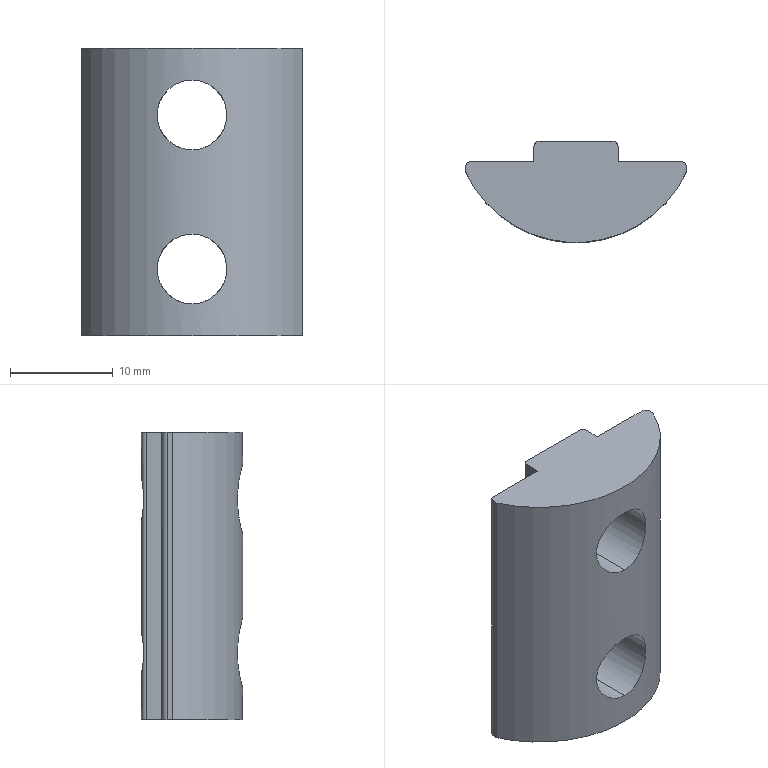Part | STEP file | 31E-01040QY25 | 1 solid | 24 faces | box 21.5 x 9.856 x 28 mm | volume 3296 mm3 | plane 11 | cylinder 9 | cone 4 | commonest cylinder face diameters 1 x4 6.8 x4 23.712 x1
STEP:
#1=CARTESIAN_POINT('',(15.532,8.15,3.1));
#2=VERTEX_POINT('',#1);
#3=CARTESIAN_POINT('',(15.532,8.15,9.9));
#4=VERTEX_POINT('',#3);
#5=CARTESIAN_POINT('',(15.532,8.15,6.5));
#6=DIRECTION('',(0.,1.,0.));
#7=AXIS2_PLACEMENT_3D('',#5,#6,$);
#8=CIRCLE('',#7,3.4);
#9=EDGE_CURVE('',#2,#4,#8,.T.);
#10=ORIENTED_EDGE('',*,*,#9,.F.);
#11=CARTESIAN_POINT('',(15.532,9.,2.25));
#12=VERTEX_POINT('',#11);
#13=CARTESIAN_POINT('',(15.532,353560.266,-353549.016));
#14=DIRECTION('',(0.,0.7071,-0.7071));
#15=VECTOR('',#14,1.);
#16=LINE('',#13,#15);
#17=EDGE_CURVE('',#2,#12,#16,.T.);
#18=ORIENTED_EDGE('',*,*,#17,.T.);
#19=CARTESIAN_POINT('',(11.932,9.,4.241));
#20=VERTEX_POINT('',#19);
#21=CARTESIAN_POINT('',(15.532,9.,6.5));
#22=DIRECTION('',(0.,1.,0.));
#23=AXIS2_PLACEMENT_3D('',#21,#22,$);
#24=CIRCLE('',#23,4.25);
#25=EDGE_CURVE('',#12,#20,#24,.T.);
#26=ORIENTED_EDGE('',*,*,#25,.T.);
#27=CARTESIAN_POINT('',(11.932,9.,8.759));
#28=VERTEX_POINT('',#27);
#29=CARTESIAN_POINT('',(11.932,9.,4.241));
#30=CARTESIAN_POINT('',(11.905,9.,4.284));
#31=CARTESIAN_POINT('',(11.88,8.998,4.329));
#32=CARTESIAN_POINT('',(11.857,8.995,4.375));
#33=CARTESIAN_POINT('',(11.806,8.986,4.483));
#34=CARTESIAN_POINT('',(11.764,8.972,4.595));
#35=CARTESIAN_POINT('',(11.743,8.964,4.654));
#36=CARTESIAN_POINT('',(11.66,8.926,4.917));
#37=CARTESIAN_POINT('',(11.605,8.884,5.186));
#38=CARTESIAN_POINT('',(11.579,8.857,5.362));
#39=CARTESIAN_POINT('',(11.542,8.815,5.679));
#40=CARTESIAN_POINT('',(11.523,8.788,5.994));
#41=CARTESIAN_POINT('',(11.518,8.781,6.11));
#42=CARTESIAN_POINT('',(11.511,8.77,6.341));
#43=CARTESIAN_POINT('',(11.511,8.769,6.572));
#44=CARTESIAN_POINT('',(11.512,8.772,6.688));
#45=CARTESIAN_POINT('',(11.521,8.785,7.009));
#46=CARTESIAN_POINT('',(11.544,8.816,7.333));
#47=CARTESIAN_POINT('',(11.566,8.844,7.546));
#48=CARTESIAN_POINT('',(11.608,8.886,7.829));
#49=CARTESIAN_POINT('',(11.674,8.929,8.111));
#50=CARTESIAN_POINT('',(11.693,8.94,8.183));
#51=CARTESIAN_POINT('',(11.741,8.964,8.344));
#52=CARTESIAN_POINT('',(11.8,8.984,8.503));
#53=CARTESIAN_POINT('',(11.839,8.994,8.595));
#54=CARTESIAN_POINT('',(11.882,9.,8.679));
#55=CARTESIAN_POINT('',(11.932,9.,8.759));
#56=B_SPLINE_CURVE_WITH_KNOTS('',5,(#29,#30,#31,#32,#33,#34,#35,#36,#37,#38,#39,#40,#41,#42,#43,#44,#45,#46,#47,#48,#49,#50,#51,#52,#53,#54,#55),.UNSPECIFIED.,.F.,.U.,(6,3,3,3,3,3,3,3,6),(0.,6.014,14.068,38.531,52.896,67.291,92.858,101.616,112.722),.UNSPECIFIED.);
#57=EDGE_CURVE('',#20,#28,#56,.T.);
#58=ORIENTED_EDGE('',*,*,#57,.T.);
#59=CARTESIAN_POINT('',(15.532,9.,10.75));
#60=VERTEX_POINT('',#59);
#61=CARTESIAN_POINT('',(15.532,9.,6.5));
#62=DIRECTION('',(0.,1.,0.));
#63=AXIS2_PLACEMENT_3D('',#61,#62,$);
#64=CIRCLE('',#63,4.25);
#65=EDGE_CURVE('',#28,#60,#64,.T.);
#66=ORIENTED_EDGE('',*,*,#65,.T.);
#67=CARTESIAN_POINT('',(15.532,353560.266,353562.016));
#68=DIRECTION('',(0.,0.7071,0.7071));
#69=VECTOR('',#68,1.);
#70=LINE('',#67,#69);
#71=EDGE_CURVE('',#4,#60,#70,.T.);
#72=ORIENTED_EDGE('',*,*,#71,.F.);
#73=EDGE_LOOP('',(#10,#18,#26,#58,#66,#72));
#74=FACE_OUTER_BOUND('',#73,.T.);
#75=CARTESIAN_POINT('',(15.532,9.,6.5));
#76=DIRECTION('',(0.,1.,0.));
#77=DIRECTION('',(0.,0.,-1.));
#78=AXIS2_PLACEMENT_3D('',#75,#76,#77);
#79=CONICAL_SURFACE('',#78,4.25,0.7854);
#80=ADVANCED_FACE('',(#74),#79,.F.);
#81=CARTESIAN_POINT('',(12.393,-0.4328,5.194));
#82=VERTEX_POINT('',#81);
#83=CARTESIAN_POINT('',(15.532,-0.8559,9.9));
#84=VERTEX_POINT('',#83);
#85=CARTESIAN_POINT('',(12.393,-0.4328,5.194));
#86=CARTESIAN_POINT('',(12.325,-0.414,5.358));
#87=CARTESIAN_POINT('',(12.267,-0.3978,5.526));
#88=CARTESIAN_POINT('',(12.221,-0.3843,5.696));
#89=CARTESIAN_POINT('',(12.151,-0.3638,6.044));
#90=CARTESIAN_POINT('',(12.126,-0.3563,6.4));
#91=CARTESIAN_POINT('',(12.126,-0.356,6.573));
#92=CARTESIAN_POINT('',(12.147,-0.3625,6.927));
#93=CARTESIAN_POINT('',(12.215,-0.3824,7.276));
#94=CARTESIAN_POINT('',(12.26,-0.3957,7.449));
#95=CARTESIAN_POINT('',(12.43,-0.4439,7.959));
#96=CARTESIAN_POINT('',(12.696,-0.5143,8.426));
#97=CARTESIAN_POINT('',(12.92,-0.5687,8.721));
#98=CARTESIAN_POINT('',(13.302,-0.6496,9.103));
#99=CARTESIAN_POINT('',(13.747,-0.7222,9.402));
#100=CARTESIAN_POINT('',(13.901,-0.7449,9.491));
#101=CARTESIAN_POINT('',(14.219,-0.7859,9.649));
#102=CARTESIAN_POINT('',(14.558,-0.8176,9.765));
#103=CARTESIAN_POINT('',(14.732,-0.8308,9.812));
#104=CARTESIAN_POINT('',(14.995,-0.8457,9.864));
#105=CARTESIAN_POINT('',(15.261,-0.8533,9.891));
#106=CARTESIAN_POINT('',(15.351,-0.855,9.897));
#107=CARTESIAN_POINT('',(15.441,-0.8559,9.9));
#108=CARTESIAN_POINT('',(15.532,-0.8559,9.9));
#109=B_SPLINE_CURVE_WITH_KNOTS('',5,(#85,#86,#87,#88,#89,#90,#91,#92,#93,#94,#95,#96,#97,#98,#99,#100,#101,#102,#103,#104,#105,#106,#107,#108),.UNSPECIFIED.,.F.,.U.,(6,3,3,3,3,3,3,6),(0.,1.257,2.514,3.773,6.322,7.596,8.853,9.491),.UNSPECIFIED.);
#110=EDGE_CURVE('',#82,#84,#109,.T.);
#111=ORIENTED_EDGE('',*,*,#110,.F.);
#112=CARTESIAN_POINT('',(15.532,-0.8559,3.1));
#113=VERTEX_POINT('',#112);
#114=CARTESIAN_POINT('',(15.532,-0.8559,3.1));
#115=CARTESIAN_POINT('',(15.357,-0.856,3.1));
#116=CARTESIAN_POINT('',(15.181,-0.8526,3.111));
#117=CARTESIAN_POINT('',(15.005,-0.8461,3.134));
#118=CARTESIAN_POINT('',(14.656,-0.8266,3.203));
#119=CARTESIAN_POINT('',(14.32,-0.7957,3.316));
#120=CARTESIAN_POINT('',(14.16,-0.7779,3.382));
#121=CARTESIAN_POINT('',(13.836,-0.7365,3.54));
#122=CARTESIAN_POINT('',(13.536,-0.6882,3.739));
#123=CARTESIAN_POINT('',(13.393,-0.6627,3.848));
#124=CARTESIAN_POINT('',(13.125,-0.6107,4.082));
#125=CARTESIAN_POINT('',(12.888,-0.5582,4.351));
#126=CARTESIAN_POINT('',(12.772,-0.5309,4.503));
#127=CARTESIAN_POINT('',(12.626,-0.4947,4.722));
#128=CARTESIAN_POINT('',(12.501,-0.4621,4.955));
#129=CARTESIAN_POINT('',(12.463,-0.4518,5.034));
#130=CARTESIAN_POINT('',(12.426,-0.442,5.113));
#131=CARTESIAN_POINT('',(12.393,-0.4328,5.194));
#132=B_SPLINE_CURVE_WITH_KNOTS('',5,(#114,#115,#116,#117,#118,#119,#120,#121,#122,#123,#124,#125,#126,#127,#128,#129,#130,#131),.UNSPECIFIED.,.F.,.U.,(6,3,3,3,3,6),(0.,1.244,2.516,3.802,5.068,5.69),.UNSPECIFIED.);
#133=EDGE_CURVE('',#113,#82,#132,.T.);
#134=ORIENTED_EDGE('',*,*,#133,.F.);
#135=CARTESIAN_POINT('',(15.532,9.,3.1));
#136=DIRECTION('',(0.,1.,0.));
#137=VECTOR('',#136,1.);
#138=LINE('',#135,#137);
#139=EDGE_CURVE('',#113,#2,#138,.T.);
#140=ORIENTED_EDGE('',*,*,#139,.T.);
#141=ORIENTED_EDGE('',*,*,#9,.T.);
#142=CARTESIAN_POINT('',(15.532,9.,9.9));
#143=DIRECTION('',(0.,1.,0.));
#144=VECTOR('',#143,1.);
#145=LINE('',#142,#144);
#146=EDGE_CURVE('',#84,#4,#145,.T.);
#147=ORIENTED_EDGE('',*,*,#146,.F.);
#148=EDGE_LOOP('',(#111,#134,#140,#141,#147));
#149=FACE_OUTER_BOUND('',#148,.T.);
#150=CARTESIAN_POINT('',(15.532,9.,6.5));
#151=DIRECTION('',(0.,1.,0.));
#152=DIRECTION('',(0.,0.,-1.));
#153=AXIS2_PLACEMENT_3D('',#150,#151,#152);
#154=CYLINDRICAL_SURFACE('',#153,3.4);
#155=ADVANCED_FACE('',(#149),#154,.F.);
#156=ORIENTED_EDGE('',*,*,#17,.F.);
#157=CARTESIAN_POINT('',(15.532,8.15,6.5));
#158=DIRECTION('',(0.,1.,0.));
#159=AXIS2_PLACEMENT_3D('',#157,#158,$);
#160=CIRCLE('',#159,3.4);
#161=EDGE_CURVE('',#4,#2,#160,.T.);
#162=ORIENTED_EDGE('',*,*,#161,.F.);
#163=ORIENTED_EDGE('',*,*,#71,.T.);
#164=CARTESIAN_POINT('',(19.132,9.,8.759));
#165=VERTEX_POINT('',#164);
#166=CARTESIAN_POINT('',(15.532,9.,6.5));
#167=DIRECTION('',(0.,1.,0.));
#168=AXIS2_PLACEMENT_3D('',#166,#167,$);
#169=CIRCLE('',#168,4.25);
#170=EDGE_CURVE('',#60,#165,#169,.T.);
#171=ORIENTED_EDGE('',*,*,#170,.T.);
#172=CARTESIAN_POINT('',(19.132,9.,4.241));
#173=VERTEX_POINT('',#172);
#174=CARTESIAN_POINT('',(19.132,9.,8.759));
#175=CARTESIAN_POINT('',(19.159,9.,8.716));
#176=CARTESIAN_POINT('',(19.184,8.998,8.671));
#177=CARTESIAN_POINT('',(19.207,8.995,8.625));
#178=CARTESIAN_POINT('',(19.258,8.986,8.517));
#179=CARTESIAN_POINT('',(19.3,8.972,8.405));
#180=CARTESIAN_POINT('',(19.321,8.964,8.346));
#181=CARTESIAN_POINT('',(19.404,8.926,8.083));
#182=CARTESIAN_POINT('',(19.459,8.884,7.814));
#183=CARTESIAN_POINT('',(19.485,8.857,7.638));
#184=CARTESIAN_POINT('',(19.522,8.815,7.321));
#185=CARTESIAN_POINT('',(19.541,8.788,7.006));
#186=CARTESIAN_POINT('',(19.546,8.781,6.89));
#187=CARTESIAN_POINT('',(19.553,8.77,6.659));
#188=CARTESIAN_POINT('',(19.553,8.769,6.428));
#189=CARTESIAN_POINT('',(19.552,8.772,6.312));
#190=CARTESIAN_POINT('',(19.543,8.785,5.991));
#191=CARTESIAN_POINT('',(19.52,8.816,5.667));
#192=CARTESIAN_POINT('',(19.498,8.844,5.454));
#193=CARTESIAN_POINT('',(19.456,8.886,5.171));
#194=CARTESIAN_POINT('',(19.39,8.929,4.889));
#195=CARTESIAN_POINT('',(19.371,8.94,4.817));
#196=CARTESIAN_POINT('',(19.323,8.964,4.656));
#197=CARTESIAN_POINT('',(19.264,8.984,4.497));
#198=CARTESIAN_POINT('',(19.225,8.994,4.405));
#199=CARTESIAN_POINT('',(19.182,9.,4.321));
#200=CARTESIAN_POINT('',(19.132,9.,4.241));
#201=B_SPLINE_CURVE_WITH_KNOTS('',5,(#174,#175,#176,#177,#178,#179,#180,#181,#182,#183,#184,#185,#186,#187,#188,#189,#190,#191,#192,#193,#194,#195,#196,#197,#198,#199,#200),.UNSPECIFIED.,.F.,.U.,(6,3,3,3,3,3,3,3,6),(0.,6.014,14.068,38.531,52.896,67.291,92.858,101.616,112.722),.UNSPECIFIED.);
#202=EDGE_CURVE('',#165,#173,#201,.T.);
#203=ORIENTED_EDGE('',*,*,#202,.T.);
#204=CARTESIAN_POINT('',(15.532,9.,6.5));
#205=DIRECTION('',(0.,1.,0.));
#206=AXIS2_PLACEMENT_3D('',#204,#205,$);
#207=CIRCLE('',#206,4.25);
#208=EDGE_CURVE('',#173,#12,#207,.T.);
#209=ORIENTED_EDGE('',*,*,#208,.T.);
#210=EDGE_LOOP('',(#156,#162,#163,#171,#203,#209));
#211=FACE_OUTER_BOUND('',#210,.T.);
#212=CARTESIAN_POINT('',(15.532,9.,6.5));
#213=DIRECTION('',(0.,1.,0.));
#214=DIRECTION('',(0.,0.,1.));
#215=AXIS2_PLACEMENT_3D('',#212,#213,#214);
#216=CONICAL_SURFACE('',#215,4.25,0.7854);
#217=ADVANCED_FACE('',(#211),#216,.F.);
#218=CARTESIAN_POINT('',(11.932,9.,0.));
#219=VERTEX_POINT('',#218);
#220=CARTESIAN_POINT('',(11.932,9.,2.121));
#221=DIRECTION('',(0.,0.,1.));
#222=VECTOR('',#221,1.);
#223=LINE('',#220,#222);
#224=EDGE_CURVE('',#219,#20,#223,.T.);
#225=ORIENTED_EDGE('',*,*,#224,.T.);
#226=ORIENTED_EDGE('',*,*,#25,.F.);
#227=ORIENTED_EDGE('',*,*,#208,.F.);
#228=CARTESIAN_POINT('',(19.132,9.,0.));
#229=VERTEX_POINT('',#228);
#230=CARTESIAN_POINT('',(19.132,9.,2.121));
#231=DIRECTION('',(0.,0.,-1.));
#232=VECTOR('',#231,1.);
#233=LINE('',#230,#232);
#234=EDGE_CURVE('',#173,#229,#233,.T.);
#235=ORIENTED_EDGE('',*,*,#234,.T.);
#236=CARTESIAN_POINT('',(15.532,9.,0.));
#237=DIRECTION('',(-1.,0.,0.));
#238=VECTOR('',#237,1.);
#239=LINE('',#236,#238);
#240=EDGE_CURVE('',#229,#219,#239,.T.);
#241=ORIENTED_EDGE('',*,*,#240,.T.);
#242=EDGE_LOOP('',(#225,#226,#227,#235,#241));
#243=FACE_OUTER_BOUND('',#242,.T.);
#244=CARTESIAN_POINT('',(11.432,9.,28.));
#245=DIRECTION('',(0.,-1.,0.));
#246=DIRECTION('',(1.,0.,0.));
#247=AXIS2_PLACEMENT_3D('',#244,#245,#246);
#248=PLANE('',#247);
#249=ADVANCED_FACE('',(#243),#248,.F.);
#250=ORIENTED_EDGE('',*,*,#57,.F.);
#251=ORIENTED_EDGE('',*,*,#224,.F.);
#252=CARTESIAN_POINT('',(11.432,8.5,0.));
#253=VERTEX_POINT('',#252);
#254=CARTESIAN_POINT('',(11.932,8.5,0.));
#255=DIRECTION('',(0.,0.,-1.));
#256=AXIS2_PLACEMENT_3D('',#254,#255,$);
#257=CIRCLE('',#256,0.5);
#258=EDGE_CURVE('',#253,#219,#257,.T.);
#259=ORIENTED_EDGE('',*,*,#258,.F.);
#260=CARTESIAN_POINT('',(11.432,8.5,28.));
#261=VERTEX_POINT('',#260);
#262=CARTESIAN_POINT('',(11.432,8.5,28.));
#263=DIRECTION('',(0.,0.,-1.));
#264=VECTOR('',#263,1.);
#265=LINE('',#262,#264);
#266=EDGE_CURVE('',#261,#253,#265,.T.);
#267=ORIENTED_EDGE('',*,*,#266,.F.);
#268=CARTESIAN_POINT('',(11.932,9.,28.));
#269=VERTEX_POINT('',#268);
#270=CARTESIAN_POINT('',(11.932,8.5,28.));
#271=DIRECTION('',(0.,0.,-1.));
#272=AXIS2_PLACEMENT_3D('',#270,#271,$);
#273=CIRCLE('',#272,0.5);
#274=EDGE_CURVE('',#269,#261,#273,.F.);
#275=ORIENTED_EDGE('',*,*,#274,.F.);
#276=CARTESIAN_POINT('',(11.932,9.,23.759));
#277=VERTEX_POINT('',#276);
#278=CARTESIAN_POINT('',(11.932,9.,28.));
#279=DIRECTION('',(0.,0.,-1.));
#280=VECTOR('',#279,1.);
#281=LINE('',#278,#280);
#282=EDGE_CURVE('',#277,#269,#281,.F.);
#283=ORIENTED_EDGE('',*,*,#282,.F.);
#284=CARTESIAN_POINT('',(11.932,9.,19.241));
#285=VERTEX_POINT('',#284);
#286=CARTESIAN_POINT('',(11.932,9.,19.241));
#287=CARTESIAN_POINT('',(11.869,9.,19.342));
#288=CARTESIAN_POINT('',(11.817,8.99,19.45));
#289=CARTESIAN_POINT('',(11.774,8.977,19.56));
#290=CARTESIAN_POINT('',(11.708,8.95,19.757));
#291=CARTESIAN_POINT('',(11.657,8.919,19.958));
#292=CARTESIAN_POINT('',(11.638,8.905,20.046));
#293=CARTESIAN_POINT('',(11.578,8.859,20.353));
#294=CARTESIAN_POINT('',(11.543,8.817,20.666));
#295=CARTESIAN_POINT('',(11.526,8.793,20.891));
#296=CARTESIAN_POINT('',(11.502,8.756,21.443));
#297=CARTESIAN_POINT('',(11.516,8.777,21.996));
#298=CARTESIAN_POINT('',(11.537,8.811,22.324));
#299=CARTESIAN_POINT('',(11.582,8.87,22.722));
#300=CARTESIAN_POINT('',(11.675,8.929,23.111));
#301=CARTESIAN_POINT('',(11.693,8.94,23.183));
#302=CARTESIAN_POINT('',(11.741,8.964,23.345));
#303=CARTESIAN_POINT('',(11.8,8.984,23.503));
#304=CARTESIAN_POINT('',(11.838,8.994,23.594));
#305=CARTESIAN_POINT('',(11.881,9.,23.678));
#306=CARTESIAN_POINT('',(11.932,9.,23.759));
#307=B_SPLINE_CURVE_WITH_KNOTS('',5,(#286,#287,#288,#289,#290,#291,#292,#293,#294,#295,#296,#297,#298,#299,#300,#301,#302,#303,#304,#305,#306),.UNSPECIFIED.,.F.,.U.,(6,3,3,3,3,3,6),(0.,0.8404,1.481,3.08,5.407,5.934,6.607),.UNSPECIFIED.);
#308=EDGE_CURVE('',#285,#277,#307,.T.);
#309=ORIENTED_EDGE('',*,*,#308,.F.);
#310=CARTESIAN_POINT('',(11.932,9.,28.));
#311=DIRECTION('',(0.,0.,-1.));
#312=VECTOR('',#311,1.);
#313=LINE('',#310,#312);
#314=EDGE_CURVE('',#28,#285,#313,.F.);
#315=ORIENTED_EDGE('',*,*,#314,.F.);
#316=EDGE_LOOP('',(#250,#251,#259,#267,#275,#283,#309,#315));
#317=FACE_OUTER_BOUND('',#316,.T.);
#318=CARTESIAN_POINT('',(11.932,8.5,28.));
#319=DIRECTION('',(0.,0.,-1.));
#320=DIRECTION('',(-1.,0.,0.));
#321=AXIS2_PLACEMENT_3D('',#318,#319,#320);
#322=CYLINDRICAL_SURFACE('',#321,0.5);
#323=ADVANCED_FACE('',(#317),#322,.T.);
#324=CARTESIAN_POINT('',(19.132,9.,19.241));
#325=VERTEX_POINT('',#324);
#326=CARTESIAN_POINT('',(19.132,9.,14.));
#327=DIRECTION('',(0.,0.,-1.));
#328=VECTOR('',#327,1.);
#329=LINE('',#326,#328);
#330=EDGE_CURVE('',#325,#165,#329,.T.);
#331=ORIENTED_EDGE('',*,*,#330,.T.);
#332=ORIENTED_EDGE('',*,*,#170,.F.);
#333=ORIENTED_EDGE('',*,*,#65,.F.);
#334=ORIENTED_EDGE('',*,*,#314,.T.);
#335=CARTESIAN_POINT('',(15.532,9.,17.25));
#336=VERTEX_POINT('',#335);
#337=CARTESIAN_POINT('',(15.532,9.,17.25));
#338=CARTESIAN_POINT('',(15.128,9.,17.25));
#339=CARTESIAN_POINT('',(14.724,9.,17.298));
#340=CARTESIAN_POINT('',(14.328,9.,17.394));
#341=CARTESIAN_POINT('',(13.565,9.,17.678));
#342=CARTESIAN_POINT('',(12.891,9.,18.133));
#343=CARTESIAN_POINT('',(12.582,9.,18.4));
#344=CARTESIAN_POINT('',(12.274,9.,18.739));
#345=CARTESIAN_POINT('',(12.015,9.,19.113));
#346=CARTESIAN_POINT('',(11.987,9.,19.155));
#347=CARTESIAN_POINT('',(11.959,9.,19.198));
#348=CARTESIAN_POINT('',(11.932,9.,19.241));
#349=B_SPLINE_CURVE_WITH_KNOTS('',5,(#337,#338,#339,#340,#341,#342,#343,#344,#345,#346,#347,#348),.UNSPECIFIED.,.F.,.U.,(6,3,3,6),(0.,2.857,5.713,6.073),.UNSPECIFIED.);
#350=EDGE_CURVE('',#336,#285,#349,.T.);
#351=ORIENTED_EDGE('',*,*,#350,.F.);
#352=CARTESIAN_POINT('',(19.132,9.,19.241));
#353=CARTESIAN_POINT('',(18.917,9.,18.899));
#354=CARTESIAN_POINT('',(18.662,9.,18.582));
#355=CARTESIAN_POINT('',(18.37,9.,18.298));
#356=CARTESIAN_POINT('',(17.724,9.,17.803));
#357=CARTESIAN_POINT('',(16.98,9.,17.473));
#358=CARTESIAN_POINT('',(16.59,9.,17.354));
#359=CARTESIAN_POINT('',(16.139,9.,17.273));
#360=CARTESIAN_POINT('',(15.685,9.,17.252));
#361=CARTESIAN_POINT('',(15.634,9.,17.251));
#362=CARTESIAN_POINT('',(15.583,9.,17.25));
#363=CARTESIAN_POINT('',(15.532,9.,17.25));
#364=B_SPLINE_CURVE_WITH_KNOTS('',5,(#352,#353,#354,#355,#356,#357,#358,#359,#360,#361,#362,#363),.UNSPECIFIED.,.F.,.U.,(6,3,3,6),(0.,2.857,5.713,6.073),.UNSPECIFIED.);
#365=EDGE_CURVE('',#325,#336,#364,.T.);
#366=ORIENTED_EDGE('',*,*,#365,.F.);
#367=EDGE_LOOP('',(#331,#332,#333,#334,#351,#366));
#368=FACE_OUTER_BOUND('',#367,.T.);
#369=CARTESIAN_POINT('',(11.432,9.,28.));
#370=DIRECTION('',(0.,-1.,0.));
#371=DIRECTION('',(1.,0.,0.));
#372=AXIS2_PLACEMENT_3D('',#369,#370,#371);
#373=PLANE('',#372);
#374=ADVANCED_FACE('',(#368),#373,.F.);
#375=CARTESIAN_POINT('',(4.782,6.,0.));
#376=VERTEX_POINT('',#375);
#377=CARTESIAN_POINT('',(26.282,6.,0.));
#378=VERTEX_POINT('',#377);
#379=CARTESIAN_POINT('',(15.532,11.,0.));
#380=DIRECTION('',(0.,0.,-1.));
#381=AXIS2_PLACEMENT_3D('',#379,#380,$);
#382=CIRCLE('',#381,11.856);
#383=EDGE_CURVE('',#376,#378,#382,.F.);
#384=ORIENTED_EDGE('',*,*,#383,.T.);
#385=CARTESIAN_POINT('',(26.282,6.,28.));
#386=VERTEX_POINT('',#385);
#387=CARTESIAN_POINT('',(26.282,6.,28.));
#388=DIRECTION('',(0.,0.,-1.));
#389=VECTOR('',#388,1.);
#390=LINE('',#387,#389);
#391=EDGE_CURVE('',#386,#378,#390,.T.);
#392=ORIENTED_EDGE('',*,*,#391,.F.);
#393=CARTESIAN_POINT('',(4.782,6.,28.));
#394=VERTEX_POINT('',#393);
#395=CARTESIAN_POINT('',(15.532,11.,28.));
#396=DIRECTION('',(0.,0.,-1.));
#397=AXIS2_PLACEMENT_3D('',#395,#396,$);
#398=CIRCLE('',#397,11.856);
#399=EDGE_CURVE('',#394,#386,#398,.F.);
#400=ORIENTED_EDGE('',*,*,#399,.F.);
#401=CARTESIAN_POINT('',(4.782,6.,28.));
#402=DIRECTION('',(0.,0.,-1.));
#403=VECTOR('',#402,1.);
#404=LINE('',#401,#403);
#405=EDGE_CURVE('',#394,#376,#404,.T.);
#406=ORIENTED_EDGE('',*,*,#405,.T.);
#407=EDGE_LOOP('',(#384,#392,#400,#406));
#408=FACE_OUTER_BOUND('',#407,.T.);
#409=CARTESIAN_POINT('',(15.532,-0.8559,24.9));
#410=VERTEX_POINT('',#409);
#411=CARTESIAN_POINT('',(18.357,-0.5143,23.391));
#412=VERTEX_POINT('',#411);
#413=CARTESIAN_POINT('',(15.532,-0.8559,24.9));
#414=CARTESIAN_POINT('',(16.207,-0.8559,24.899));
#415=CARTESIAN_POINT('',(16.868,-0.8088,24.737));
#416=CARTESIAN_POINT('',(17.489,-0.7125,24.4));
#417=CARTESIAN_POINT('',(17.986,-0.6055,23.946));
#418=CARTESIAN_POINT('',(18.357,-0.5143,23.391));
#419=B_SPLINE_CURVE_WITH_KNOTS('',5,(#413,#414,#415,#416,#417,#418),.UNSPECIFIED.,.F.,.U.,(6,6),(0.,4.749),.UNSPECIFIED.);
#420=EDGE_CURVE('',#410,#412,#419,.T.);
#421=ORIENTED_EDGE('',*,*,#420,.T.);
#422=CARTESIAN_POINT('',(15.532,-0.8559,18.1));
#423=VERTEX_POINT('',#422);
#424=CARTESIAN_POINT('',(18.357,-0.5143,23.391));
#425=CARTESIAN_POINT('',(18.555,-0.4658,23.096));
#426=CARTESIAN_POINT('',(18.713,-0.4225,22.778));
#427=CARTESIAN_POINT('',(18.83,-0.3884,22.437));
#428=CARTESIAN_POINT('',(18.935,-0.3569,21.911));
#429=CARTESIAN_POINT('',(18.937,-0.3566,21.377));
#430=CARTESIAN_POINT('',(18.925,-0.3599,21.198));
#431=CARTESIAN_POINT('',(18.88,-0.3734,20.846));
#432=CARTESIAN_POINT('',(18.79,-0.3996,20.504));
#433=CARTESIAN_POINT('',(18.733,-0.4158,20.335));
#434=CARTESIAN_POINT('',(18.598,-0.4532,20.005));
#435=CARTESIAN_POINT('',(18.422,-0.4989,19.695));
#436=CARTESIAN_POINT('',(18.324,-0.5233,19.547));
#437=CARTESIAN_POINT('',(18.106,-0.5747,19.261));
#438=CARTESIAN_POINT('',(17.853,-0.6276,19.006));
#439=CARTESIAN_POINT('',(17.719,-0.6538,18.887));
#440=CARTESIAN_POINT('',(17.26,-0.7359,18.533));
#441=CARTESIAN_POINT('',(16.728,-0.8046,18.28));
#442=CARTESIAN_POINT('',(16.341,-0.8389,18.162));
#443=CARTESIAN_POINT('',(15.934,-0.8559,18.1));
#444=CARTESIAN_POINT('',(15.532,-0.8559,18.1));
#445=B_SPLINE_CURVE_WITH_KNOTS('',5,(#424,#425,#426,#427,#428,#429,#430,#431,#432,#433,#434,#435,#436,#437,#438,#439,#440,#441,#442,#443,#444),.UNSPECIFIED.,.F.,.U.,(6,3,3,3,3,3,6),(0.,2.528,3.777,5.033,6.311,7.596,10.449),.UNSPECIFIED.);
#446=EDGE_CURVE('',#412,#423,#445,.T.);
#447=ORIENTED_EDGE('',*,*,#446,.T.);
#448=CARTESIAN_POINT('',(12.393,-0.4328,20.194));
#449=VERTEX_POINT('',#448);
#450=CARTESIAN_POINT('',(15.532,-0.8559,18.1));
#451=CARTESIAN_POINT('',(15.357,-0.8559,18.1));
#452=CARTESIAN_POINT('',(15.181,-0.8527,18.111));
#453=CARTESIAN_POINT('',(15.005,-0.8461,18.134));
#454=CARTESIAN_POINT('',(14.657,-0.8267,18.203));
#455=CARTESIAN_POINT('',(14.322,-0.7958,18.315));
#456=CARTESIAN_POINT('',(14.158,-0.7777,18.382));
#457=CARTESIAN_POINT('',(13.835,-0.7364,18.541));
#458=CARTESIAN_POINT('',(13.536,-0.6882,18.739));
#459=CARTESIAN_POINT('',(13.393,-0.6627,18.847));
#460=CARTESIAN_POINT('',(13.058,-0.5977,19.141));
#461=CARTESIAN_POINT('',(12.772,-0.532,19.488));
#462=CARTESIAN_POINT('',(12.622,-0.4944,19.711));
#463=CARTESIAN_POINT('',(12.496,-0.4611,19.946));
#464=CARTESIAN_POINT('',(12.393,-0.4328,20.194));
#465=B_SPLINE_CURVE_WITH_KNOTS('',5,(#450,#451,#452,#453,#454,#455,#456,#457,#458,#459,#460,#461,#462,#463,#464),.UNSPECIFIED.,.F.,.U.,(6,3,3,3,6),(0.,1.244,2.51,3.797,5.701),.UNSPECIFIED.);
#466=EDGE_CURVE('',#423,#449,#465,.T.);
#467=ORIENTED_EDGE('',*,*,#466,.T.);
#468=CARTESIAN_POINT('',(12.393,-0.4328,20.194));
#469=CARTESIAN_POINT('',(12.325,-0.414,20.358));
#470=CARTESIAN_POINT('',(12.267,-0.3977,20.526));
#471=CARTESIAN_POINT('',(12.221,-0.3843,20.696));
#472=CARTESIAN_POINT('',(12.151,-0.3638,21.043));
#473=CARTESIAN_POINT('',(12.127,-0.3564,21.398));
#474=CARTESIAN_POINT('',(12.126,-0.3561,21.574));
#475=CARTESIAN_POINT('',(12.147,-0.3625,21.928));
#476=CARTESIAN_POINT('',(12.215,-0.3824,22.276));
#477=CARTESIAN_POINT('',(12.26,-0.3957,22.449));
#478=CARTESIAN_POINT('',(12.431,-0.4443,22.961));
#479=CARTESIAN_POINT('',(12.698,-0.5147,23.43));
#480=CARTESIAN_POINT('',(12.918,-0.5681,23.718));
#481=CARTESIAN_POINT('',(13.3,-0.6495,24.102));
#482=CARTESIAN_POINT('',(13.747,-0.7222,24.402));
#483=CARTESIAN_POINT('',(13.901,-0.7448,24.492));
#484=CARTESIAN_POINT('',(14.3,-0.7963,24.689));
#485=CARTESIAN_POINT('',(14.731,-0.8332,24.82));
#486=CARTESIAN_POINT('',(14.995,-0.8483,24.874));
#487=CARTESIAN_POINT('',(15.263,-0.8559,24.9));
#488=CARTESIAN_POINT('',(15.532,-0.8559,24.9));
#489=B_SPLINE_CURVE_WITH_KNOTS('',5,(#468,#469,#470,#471,#472,#473,#474,#475,#476,#477,#478,#479,#480,#481,#482,#483,#484,#485,#486,#487,#488),.UNSPECIFIED.,.F.,.U.,(6,3,3,3,3,3,6),(0.,1.258,2.509,3.766,6.328,7.603,9.5),.UNSPECIFIED.);
#490=EDGE_CURVE('',#449,#410,#489,.T.);
#491=ORIENTED_EDGE('',*,*,#490,.T.);
#492=EDGE_LOOP('',(#421,#447,#467,#491));
#493=FACE_BOUND('',#492,.T.);
#494=CARTESIAN_POINT('',(18.357,-0.5143,8.391));
#495=VERTEX_POINT('',#494);
#496=CARTESIAN_POINT('',(15.532,-0.8559,9.9));
#497=CARTESIAN_POINT('',(16.207,-0.8559,9.899));
#498=CARTESIAN_POINT('',(16.868,-0.8088,9.737));
#499=CARTESIAN_POINT('',(17.489,-0.7125,9.4));
#500=CARTESIAN_POINT('',(17.986,-0.6055,8.946));
#501=CARTESIAN_POINT('',(18.357,-0.5143,8.391));
#502=B_SPLINE_CURVE_WITH_KNOTS('',5,(#496,#497,#498,#499,#500,#501),.UNSPECIFIED.,.F.,.U.,(6,6),(0.,4.749),.UNSPECIFIED.);
#503=EDGE_CURVE('',#84,#495,#502,.T.);
#504=ORIENTED_EDGE('',*,*,#503,.T.);
#505=CARTESIAN_POINT('',(18.357,-0.5143,8.391));
#506=CARTESIAN_POINT('',(18.555,-0.4658,8.096));
#507=CARTESIAN_POINT('',(18.713,-0.4225,7.778));
#508=CARTESIAN_POINT('',(18.83,-0.3884,7.437));
#509=CARTESIAN_POINT('',(18.935,-0.3569,6.911));
#510=CARTESIAN_POINT('',(18.937,-0.3566,6.377));
#511=CARTESIAN_POINT('',(18.925,-0.3599,6.198));
#512=CARTESIAN_POINT('',(18.88,-0.3734,5.846));
#513=CARTESIAN_POINT('',(18.79,-0.3996,5.504));
#514=CARTESIAN_POINT('',(18.733,-0.4158,5.335));
#515=CARTESIAN_POINT('',(18.598,-0.4532,5.005));
#516=CARTESIAN_POINT('',(18.422,-0.4989,4.695));
#517=CARTESIAN_POINT('',(18.324,-0.5233,4.547));
#518=CARTESIAN_POINT('',(18.106,-0.5747,4.261));
#519=CARTESIAN_POINT('',(17.853,-0.6276,4.006));
#520=CARTESIAN_POINT('',(17.719,-0.6538,3.887));
#521=CARTESIAN_POINT('',(17.26,-0.7359,3.533));
#522=CARTESIAN_POINT('',(16.728,-0.8046,3.28));
#523=CARTESIAN_POINT('',(16.341,-0.8389,3.162));
#524=CARTESIAN_POINT('',(15.934,-0.8559,3.1));
#525=CARTESIAN_POINT('',(15.532,-0.8559,3.1));
#526=B_SPLINE_CURVE_WITH_KNOTS('',5,(#505,#506,#507,#508,#509,#510,#511,#512,#513,#514,#515,#516,#517,#518,#519,#520,#521,#522,#523,#524,#525),.UNSPECIFIED.,.F.,.U.,(6,3,3,3,3,3,6),(0.,2.528,3.777,5.033,6.311,7.596,10.449),.UNSPECIFIED.);
#527=EDGE_CURVE('',#495,#113,#526,.T.);
#528=ORIENTED_EDGE('',*,*,#527,.T.);
#529=ORIENTED_EDGE('',*,*,#133,.T.);
#530=ORIENTED_EDGE('',*,*,#110,.T.);
#531=EDGE_LOOP('',(#504,#528,#529,#530));
#532=FACE_BOUND('',#531,.T.);
#533=CARTESIAN_POINT('',(15.532,11.,28.));
#534=DIRECTION('',(0.,0.,-1.));
#535=DIRECTION('',(1.,0.,0.));
#536=AXIS2_PLACEMENT_3D('',#533,#534,#535);
#537=CYLINDRICAL_SURFACE('',#536,11.856);
#538=ADVANCED_FACE('',(#408,#493,#532),#537,.T.);
#539=ORIENTED_EDGE('',*,*,#139,.F.);
#540=ORIENTED_EDGE('',*,*,#527,.F.);
#541=ORIENTED_EDGE('',*,*,#503,.F.);
#542=ORIENTED_EDGE('',*,*,#146,.T.);
#543=ORIENTED_EDGE('',*,*,#161,.T.);
#544=EDGE_LOOP('',(#539,#540,#541,#542,#543));
#545=FACE_OUTER_BOUND('',#544,.T.);
#546=CARTESIAN_POINT('',(15.532,9.,6.5));
#547=DIRECTION('',(0.,1.,0.));
#548=DIRECTION('',(0.,0.,1.));
#549=AXIS2_PLACEMENT_3D('',#546,#547,#548);
#550=CYLINDRICAL_SURFACE('',#549,3.4);
#551=ADVANCED_FACE('',(#545),#550,.F.);
#552=ORIENTED_EDGE('',*,*,#202,.F.);
#553=ORIENTED_EDGE('',*,*,#330,.F.);
#554=CARTESIAN_POINT('',(19.132,9.,23.759));
#555=VERTEX_POINT('',#554);
#556=CARTESIAN_POINT('',(19.132,9.,23.759));
#557=CARTESIAN_POINT('',(19.195,9.,23.658));
#558=CARTESIAN_POINT('',(19.247,8.99,23.55));
#559=CARTESIAN_POINT('',(19.29,8.977,23.44));
#560=CARTESIAN_POINT('',(19.356,8.95,23.243));
#561=CARTESIAN_POINT('',(19.407,8.919,23.042));
#562=CARTESIAN_POINT('',(19.426,8.905,22.954));
#563=CARTESIAN_POINT('',(19.486,8.859,22.647));
#564=CARTESIAN_POINT('',(19.521,8.817,22.334));
#565=CARTESIAN_POINT('',(19.538,8.793,22.109));
#566=CARTESIAN_POINT('',(19.562,8.756,21.557));
#567=CARTESIAN_POINT('',(19.548,8.777,21.004));
#568=CARTESIAN_POINT('',(19.527,8.811,20.676));
#569=CARTESIAN_POINT('',(19.482,8.87,20.278));
#570=CARTESIAN_POINT('',(19.389,8.929,19.889));
#571=CARTESIAN_POINT('',(19.371,8.94,19.817));
#572=CARTESIAN_POINT('',(19.323,8.964,19.655));
#573=CARTESIAN_POINT('',(19.264,8.984,19.497));
#574=CARTESIAN_POINT('',(19.226,8.994,19.406));
#575=CARTESIAN_POINT('',(19.183,9.,19.322));
#576=CARTESIAN_POINT('',(19.132,9.,19.241));
#577=B_SPLINE_CURVE_WITH_KNOTS('',5,(#556,#557,#558,#559,#560,#561,#562,#563,#564,#565,#566,#567,#568,#569,#570,#571,#572,#573,#574,#575,#576),.UNSPECIFIED.,.F.,.U.,(6,3,3,3,3,3,6),(0.,0.8404,1.481,3.08,5.407,5.934,6.607),.UNSPECIFIED.);
#578=EDGE_CURVE('',#555,#325,#577,.T.);
#579=ORIENTED_EDGE('',*,*,#578,.F.);
#580=CARTESIAN_POINT('',(19.132,9.,28.));
#581=VERTEX_POINT('',#580);
#582=CARTESIAN_POINT('',(19.132,9.,28.));
#583=DIRECTION('',(0.,0.,-1.));
#584=VECTOR('',#583,1.);
#585=LINE('',#582,#584);
#586=EDGE_CURVE('',#581,#555,#585,.T.);
#587=ORIENTED_EDGE('',*,*,#586,.F.);
#588=CARTESIAN_POINT('',(19.632,8.5,28.));
#589=VERTEX_POINT('',#588);
#590=CARTESIAN_POINT('',(19.132,8.5,28.));
#591=DIRECTION('',(0.,0.,-1.));
#592=AXIS2_PLACEMENT_3D('',#590,#591,$);
#593=CIRCLE('',#592,0.5);
#594=EDGE_CURVE('',#589,#581,#593,.F.);
#595=ORIENTED_EDGE('',*,*,#594,.F.);
#596=CARTESIAN_POINT('',(19.632,8.5,0.));
#597=VERTEX_POINT('',#596);
#598=CARTESIAN_POINT('',(19.632,8.5,28.));
#599=DIRECTION('',(0.,0.,-1.));
#600=VECTOR('',#599,1.);
#601=LINE('',#598,#600);
#602=EDGE_CURVE('',#597,#589,#601,.F.);
#603=ORIENTED_EDGE('',*,*,#602,.F.);
#604=CARTESIAN_POINT('',(19.132,8.5,0.));
#605=DIRECTION('',(0.,0.,-1.));
#606=AXIS2_PLACEMENT_3D('',#604,#605,$);
#607=CIRCLE('',#606,0.5);
#608=EDGE_CURVE('',#229,#597,#607,.T.);
#609=ORIENTED_EDGE('',*,*,#608,.F.);
#610=ORIENTED_EDGE('',*,*,#234,.F.);
#611=EDGE_LOOP('',(#552,#553,#579,#587,#595,#603,#609,#610));
#612=FACE_OUTER_BOUND('',#611,.T.);
#613=CARTESIAN_POINT('',(19.132,8.5,28.));
#614=DIRECTION('',(0.,0.,-1.));
#615=DIRECTION('',(-1.,0.,0.));
#616=AXIS2_PLACEMENT_3D('',#613,#614,#615);
#617=CYLINDRICAL_SURFACE('',#616,0.5);
#618=ADVANCED_FACE('',(#612),#617,.T.);
#619=CARTESIAN_POINT('',(25.782,7.,0.));
#620=VERTEX_POINT('',#619);
#621=CARTESIAN_POINT('',(19.632,7.,0.));
#622=VERTEX_POINT('',#621);
#623=CARTESIAN_POINT('',(22.707,7.,0.));
#624=DIRECTION('',(-1.,0.,0.));
#625=VECTOR('',#624,1.);
#626=LINE('',#623,#625);
#627=EDGE_CURVE('',#620,#622,#626,.T.);
#628=ORIENTED_EDGE('',*,*,#627,.F.);
#629=CARTESIAN_POINT('',(26.282,6.5,0.));
#630=VERTEX_POINT('',#629);
#631=CARTESIAN_POINT('',(25.782,7.,0.));
#632=CARTESIAN_POINT('',(25.845,7.,0.));
#633=CARTESIAN_POINT('',(25.908,6.99,0.));
#634=CARTESIAN_POINT('',(25.968,6.97,0.));
#635=CARTESIAN_POINT('',(26.082,6.912,0.));
#636=CARTESIAN_POINT('',(26.172,6.823,0.));
#637=CARTESIAN_POINT('',(26.209,6.771,0.));
#638=CARTESIAN_POINT('',(26.252,6.686,0.));
#639=CARTESIAN_POINT('',(26.275,6.594,0.));
#640=CARTESIAN_POINT('',(26.28,6.563,0.));
#641=CARTESIAN_POINT('',(26.282,6.531,0.));
#642=CARTESIAN_POINT('',(26.282,6.5,0.));
#643=B_SPLINE_CURVE_WITH_KNOTS('',5,(#631,#632,#633,#634,#635,#636,#637,#638,#639,#640,#641,#642),.UNSPECIFIED.,.F.,.U.,(6,3,3,6),(0.,0.4443,0.8886,1.11),.UNSPECIFIED.);
#644=EDGE_CURVE('',#620,#630,#643,.T.);
#645=ORIENTED_EDGE('',*,*,#644,.T.);
#646=CARTESIAN_POINT('',(26.282,6.25,0.));
#647=DIRECTION('',(0.,1.,0.));
#648=VECTOR('',#647,1.);
#649=LINE('',#646,#648);
#650=EDGE_CURVE('',#378,#630,#649,.T.);
#651=ORIENTED_EDGE('',*,*,#650,.F.);
#652=ORIENTED_EDGE('',*,*,#383,.F.);
#653=CARTESIAN_POINT('',(4.782,6.5,0.));
#654=VERTEX_POINT('',#653);
#655=CARTESIAN_POINT('',(4.782,6.25,0.));
#656=DIRECTION('',(0.,-1.,0.));
#657=VECTOR('',#656,1.);
#658=LINE('',#655,#657);
#659=EDGE_CURVE('',#654,#376,#658,.T.);
#660=ORIENTED_EDGE('',*,*,#659,.F.);
#661=CARTESIAN_POINT('',(5.282,7.,0.));
#662=VERTEX_POINT('',#661);
#663=CARTESIAN_POINT('',(4.782,6.5,0.));
#664=CARTESIAN_POINT('',(4.782,6.563,0.));
#665=CARTESIAN_POINT('',(4.792,6.626,0.));
#666=CARTESIAN_POINT('',(4.812,6.686,0.));
#667=CARTESIAN_POINT('',(4.87,6.8,0.));
#668=CARTESIAN_POINT('',(4.959,6.89,0.));
#669=CARTESIAN_POINT('',(5.011,6.927,0.));
#670=CARTESIAN_POINT('',(5.096,6.97,0.));
#671=CARTESIAN_POINT('',(5.188,6.993,0.));
#672=CARTESIAN_POINT('',(5.219,6.998,0.));
#673=CARTESIAN_POINT('',(5.251,7.,0.));
#674=CARTESIAN_POINT('',(5.282,7.,0.));
#675=B_SPLINE_CURVE_WITH_KNOTS('',5,(#663,#664,#665,#666,#667,#668,#669,#670,#671,#672,#673,#674),.UNSPECIFIED.,.F.,.U.,(6,3,3,6),(0.,0.4443,0.8886,1.11),.UNSPECIFIED.);
#676=EDGE_CURVE('',#654,#662,#675,.T.);
#677=ORIENTED_EDGE('',*,*,#676,.T.);
#678=CARTESIAN_POINT('',(11.432,7.,0.));
#679=VERTEX_POINT('',#678);
#680=CARTESIAN_POINT('',(8.357,7.,0.));
#681=DIRECTION('',(-1.,0.,0.));
#682=VECTOR('',#681,1.);
#683=LINE('',#680,#682);
#684=EDGE_CURVE('',#679,#662,#683,.T.);
#685=ORIENTED_EDGE('',*,*,#684,.F.);
#686=CARTESIAN_POINT('',(11.432,7.75,0.));
#687=DIRECTION('',(0.,-1.,0.));
#688=VECTOR('',#687,1.);
#689=LINE('',#686,#688);
#690=EDGE_CURVE('',#253,#679,#689,.T.);
#691=ORIENTED_EDGE('',*,*,#690,.F.);
#692=ORIENTED_EDGE('',*,*,#258,.T.);
#693=ORIENTED_EDGE('',*,*,#240,.F.);
#694=ORIENTED_EDGE('',*,*,#608,.T.);
#695=CARTESIAN_POINT('',(19.632,7.75,0.));
#696=DIRECTION('',(0.,1.,0.));
#697=VECTOR('',#696,1.);
#698=LINE('',#695,#697);
#699=EDGE_CURVE('',#622,#597,#698,.T.);
#700=ORIENTED_EDGE('',*,*,#699,.F.);
#701=EDGE_LOOP('',(#628,#645,#651,#652,#660,#677,#685,#691,#692,#693,#694,#700));
#702=FACE_OUTER_BOUND('',#701,.T.);
#703=CARTESIAN_POINT('',(15.532,11.,0.));
#704=DIRECTION('',(0.,0.,1.));
#705=DIRECTION('',(1.,0.,0.));
#706=AXIS2_PLACEMENT_3D('',#703,#704,#705);
#707=PLANE('',#706);
#708=ADVANCED_FACE('',(#702),#707,.F.);
#709=CARTESIAN_POINT('',(11.432,7.,28.));
#710=VERTEX_POINT('',#709);
#711=CARTESIAN_POINT('',(11.432,7.75,28.));
#712=DIRECTION('',(0.,-1.,0.));
#713=VECTOR('',#712,1.);
#714=LINE('',#711,#713);
#715=EDGE_CURVE('',#261,#710,#714,.T.);
#716=ORIENTED_EDGE('',*,*,#715,.F.);
#717=ORIENTED_EDGE('',*,*,#266,.T.);
#718=ORIENTED_EDGE('',*,*,#690,.T.);
#719=CARTESIAN_POINT('',(11.432,7.,14.));
#720=DIRECTION('',(0.,0.,-1.));
#721=VECTOR('',#720,1.);
#722=LINE('',#719,#721);
#723=EDGE_CURVE('',#710,#679,#722,.T.);
#724=ORIENTED_EDGE('',*,*,#723,.F.);
#725=EDGE_LOOP('',(#716,#717,#718,#724));
#726=FACE_OUTER_BOUND('',#725,.T.);
#727=CARTESIAN_POINT('',(11.432,7.,28.));
#728=DIRECTION('',(1.,0.,0.));
#729=DIRECTION('',(0.,0.,-1.));
#730=AXIS2_PLACEMENT_3D('',#727,#728,#729);
#731=PLANE('',#730);
#732=ADVANCED_FACE('',(#726),#731,.F.);
#733=CARTESIAN_POINT('',(26.282,6.5,28.));
#734=VERTEX_POINT('',#733);
#735=CARTESIAN_POINT('',(26.282,6.25,28.));
#736=DIRECTION('',(0.,1.,0.));
#737=VECTOR('',#736,1.);
#738=LINE('',#735,#737);
#739=EDGE_CURVE('',#386,#734,#738,.T.);
#740=ORIENTED_EDGE('',*,*,#739,.T.);
#741=CARTESIAN_POINT('',(25.782,7.,28.));
#742=VERTEX_POINT('',#741);
#743=CARTESIAN_POINT('',(25.782,6.5,28.));
#744=DIRECTION('',(0.,0.,1.));
#745=AXIS2_PLACEMENT_3D('',#743,#744,$);
#746=CIRCLE('',#745,0.5);
#747=EDGE_CURVE('',#734,#742,#746,.T.);
#748=ORIENTED_EDGE('',*,*,#747,.T.);
#749=CARTESIAN_POINT('',(19.632,7.,28.));
#750=VERTEX_POINT('',#749);
#751=CARTESIAN_POINT('',(22.707,7.,28.));
#752=DIRECTION('',(-1.,0.,0.));
#753=VECTOR('',#752,1.);
#754=LINE('',#751,#753);
#755=EDGE_CURVE('',#742,#750,#754,.T.);
#756=ORIENTED_EDGE('',*,*,#755,.T.);
#757=CARTESIAN_POINT('',(19.632,7.75,28.));
#758=DIRECTION('',(0.,1.,0.));
#759=VECTOR('',#758,1.);
#760=LINE('',#757,#759);
#761=EDGE_CURVE('',#750,#589,#760,.T.);
#762=ORIENTED_EDGE('',*,*,#761,.T.);
#763=ORIENTED_EDGE('',*,*,#594,.T.);
#764=CARTESIAN_POINT('',(15.532,9.,28.));
#765=DIRECTION('',(-1.,0.,0.));
#766=VECTOR('',#765,1.);
#767=LINE('',#764,#766);
#768=EDGE_CURVE('',#581,#269,#767,.T.);
#769=ORIENTED_EDGE('',*,*,#768,.T.);
#770=ORIENTED_EDGE('',*,*,#274,.T.);
#771=ORIENTED_EDGE('',*,*,#715,.T.);
#772=CARTESIAN_POINT('',(5.282,7.,28.));
#773=VERTEX_POINT('',#772);
#774=CARTESIAN_POINT('',(8.357,7.,28.));
#775=DIRECTION('',(-1.,0.,0.));
#776=VECTOR('',#775,1.);
#777=LINE('',#774,#776);
#778=EDGE_CURVE('',#710,#773,#777,.T.);
#779=ORIENTED_EDGE('',*,*,#778,.T.);
#780=CARTESIAN_POINT('',(4.782,6.5,28.));
#781=VERTEX_POINT('',#780);
#782=CARTESIAN_POINT('',(5.282,6.5,28.));
#783=DIRECTION('',(0.,0.,1.));
#784=AXIS2_PLACEMENT_3D('',#782,#783,$);
#785=CIRCLE('',#784,0.5);
#786=EDGE_CURVE('',#773,#781,#785,.T.);
#787=ORIENTED_EDGE('',*,*,#786,.T.);
#788=CARTESIAN_POINT('',(4.782,6.25,28.));
#789=DIRECTION('',(0.,-1.,0.));
#790=VECTOR('',#789,1.);
#791=LINE('',#788,#790);
#792=EDGE_CURVE('',#781,#394,#791,.T.);
#793=ORIENTED_EDGE('',*,*,#792,.T.);
#794=ORIENTED_EDGE('',*,*,#399,.T.);
#795=EDGE_LOOP('',(#740,#748,#756,#762,#763,#769,#770,#771,#779,#787,#793,#794));
#796=FACE_OUTER_BOUND('',#795,.T.);
#797=CARTESIAN_POINT('',(15.532,11.,28.));
#798=DIRECTION('',(0.,0.,1.));
#799=DIRECTION('',(1.,0.,0.));
#800=AXIS2_PLACEMENT_3D('',#797,#798,#799);
#801=PLANE('',#800);
#802=ADVANCED_FACE('',(#796),#801,.T.);
#803=CARTESIAN_POINT('',(15.532,9.,25.75));
#804=VERTEX_POINT('',#803);
#805=CARTESIAN_POINT('',(11.932,9.,23.759));
#806=CARTESIAN_POINT('',(12.147,9.,24.101));
#807=CARTESIAN_POINT('',(12.402,9.,24.418));
#808=CARTESIAN_POINT('',(12.694,9.,24.702));
#809=CARTESIAN_POINT('',(13.34,9.,25.197));
#810=CARTESIAN_POINT('',(14.084,9.,25.527));
#811=CARTESIAN_POINT('',(14.474,9.,25.646));
#812=CARTESIAN_POINT('',(14.925,9.,25.727));
#813=CARTESIAN_POINT('',(15.379,9.,25.748));
#814=CARTESIAN_POINT('',(15.43,9.,25.749));
#815=CARTESIAN_POINT('',(15.481,9.,25.75));
#816=CARTESIAN_POINT('',(15.532,9.,25.75));
#817=B_SPLINE_CURVE_WITH_KNOTS('',5,(#805,#806,#807,#808,#809,#810,#811,#812,#813,#814,#815,#816),.UNSPECIFIED.,.F.,.U.,(6,3,3,6),(0.,2.857,5.713,6.073),.UNSPECIFIED.);
#818=EDGE_CURVE('',#277,#804,#817,.T.);
#819=ORIENTED_EDGE('',*,*,#818,.F.);
#820=ORIENTED_EDGE('',*,*,#282,.T.);
#821=ORIENTED_EDGE('',*,*,#768,.F.);
#822=ORIENTED_EDGE('',*,*,#586,.T.);
#823=CARTESIAN_POINT('',(15.532,9.,25.75));
#824=CARTESIAN_POINT('',(15.936,9.,25.75));
#825=CARTESIAN_POINT('',(16.34,9.,25.702));
#826=CARTESIAN_POINT('',(16.736,9.,25.606));
#827=CARTESIAN_POINT('',(17.499,9.,25.322));
#828=CARTESIAN_POINT('',(18.173,9.,24.867));
#829=CARTESIAN_POINT('',(18.482,9.,24.6));
#830=CARTESIAN_POINT('',(18.79,9.,24.261));
#831=CARTESIAN_POINT('',(19.049,9.,23.887));
#832=CARTESIAN_POINT('',(19.077,9.,23.845));
#833=CARTESIAN_POINT('',(19.105,9.,23.802));
#834=CARTESIAN_POINT('',(19.132,9.,23.759));
#835=B_SPLINE_CURVE_WITH_KNOTS('',5,(#823,#824,#825,#826,#827,#828,#829,#830,#831,#832,#833,#834),.UNSPECIFIED.,.F.,.U.,(6,3,3,6),(0.,2.857,5.713,6.073),.UNSPECIFIED.);
#836=EDGE_CURVE('',#804,#555,#835,.T.);
#837=ORIENTED_EDGE('',*,*,#836,.F.);
#838=EDGE_LOOP('',(#819,#820,#821,#822,#837));
#839=FACE_OUTER_BOUND('',#838,.T.);
#840=CARTESIAN_POINT('',(11.432,9.,28.));
#841=DIRECTION('',(0.,-1.,0.));
#842=DIRECTION('',(1.,0.,0.));
#843=AXIS2_PLACEMENT_3D('',#840,#841,#842);
#844=PLANE('',#843);
#845=ADVANCED_FACE('',(#839),#844,.F.);
#846=CARTESIAN_POINT('',(15.532,8.15,18.1));
#847=VERTEX_POINT('',#846);
#848=CARTESIAN_POINT('',(15.532,8.15,24.9));
#849=VERTEX_POINT('',#848);
#850=CARTESIAN_POINT('',(15.532,8.15,21.5));
#851=DIRECTION('',(0.,1.,0.));
#852=AXIS2_PLACEMENT_3D('',#850,#851,$);
#853=CIRCLE('',#852,3.4);
#854=EDGE_CURVE('',#847,#849,#853,.T.);
#855=ORIENTED_EDGE('',*,*,#854,.F.);
#856=CARTESIAN_POINT('',(15.532,353560.266,-353534.016));
#857=DIRECTION('',(0.,0.7071,-0.7071));
#858=VECTOR('',#857,1.);
#859=LINE('',#856,#858);
#860=EDGE_CURVE('',#847,#336,#859,.T.);
#861=ORIENTED_EDGE('',*,*,#860,.T.);
#862=ORIENTED_EDGE('',*,*,#350,.T.);
#863=ORIENTED_EDGE('',*,*,#308,.T.);
#864=ORIENTED_EDGE('',*,*,#818,.T.);
#865=CARTESIAN_POINT('',(15.532,353560.266,353577.016));
#866=DIRECTION('',(0.,0.7071,0.7071));
#867=VECTOR('',#866,1.);
#868=LINE('',#865,#867);
#869=EDGE_CURVE('',#849,#804,#868,.T.);
#870=ORIENTED_EDGE('',*,*,#869,.F.);
#871=EDGE_LOOP('',(#855,#861,#862,#863,#864,#870));
#872=FACE_OUTER_BOUND('',#871,.T.);
#873=CARTESIAN_POINT('',(15.532,9.,21.5));
#874=DIRECTION('',(0.,1.,0.));
#875=DIRECTION('',(0.,0.,-1.));
#876=AXIS2_PLACEMENT_3D('',#873,#874,#875);
#877=CONICAL_SURFACE('',#876,4.25,0.7854);
#878=ADVANCED_FACE('',(#872),#877,.F.);
#879=ORIENTED_EDGE('',*,*,#860,.F.);
#880=CARTESIAN_POINT('',(15.532,8.15,21.5));
#881=DIRECTION('',(0.,1.,0.));
#882=AXIS2_PLACEMENT_3D('',#880,#881,$);
#883=CIRCLE('',#882,3.4);
#884=EDGE_CURVE('',#849,#847,#883,.T.);
#885=ORIENTED_EDGE('',*,*,#884,.F.);
#886=ORIENTED_EDGE('',*,*,#869,.T.);
#887=ORIENTED_EDGE('',*,*,#836,.T.);
#888=ORIENTED_EDGE('',*,*,#578,.T.);
#889=ORIENTED_EDGE('',*,*,#365,.T.);
#890=EDGE_LOOP('',(#879,#885,#886,#887,#888,#889));
#891=FACE_OUTER_BOUND('',#890,.T.);
#892=CARTESIAN_POINT('',(15.532,9.,21.5));
#893=DIRECTION('',(0.,1.,0.));
#894=DIRECTION('',(0.,0.,1.));
#895=AXIS2_PLACEMENT_3D('',#892,#893,#894);
#896=CONICAL_SURFACE('',#895,4.25,0.7854);
#897=ADVANCED_FACE('',(#891),#896,.F.);
#898=ORIENTED_EDGE('',*,*,#650,.T.);
#899=CARTESIAN_POINT('',(26.282,6.5,14.));
#900=DIRECTION('',(0.,0.,1.));
#901=VECTOR('',#900,1.);
#902=LINE('',#899,#901);
#903=EDGE_CURVE('',#630,#734,#902,.T.);
#904=ORIENTED_EDGE('',*,*,#903,.T.);
#905=ORIENTED_EDGE('',*,*,#739,.F.);
#906=ORIENTED_EDGE('',*,*,#391,.T.);
#907=EDGE_LOOP('',(#898,#904,#905,#906));
#908=FACE_OUTER_BOUND('',#907,.T.);
#909=CARTESIAN_POINT('',(26.282,6.,28.));
#910=DIRECTION('',(-1.,0.,0.));
#911=DIRECTION('',(0.,-1.,0.));
#912=AXIS2_PLACEMENT_3D('',#909,#910,#911);
#913=PLANE('',#912);
#914=ADVANCED_FACE('',(#908),#913,.F.);
#915=ORIENTED_EDGE('',*,*,#792,.F.);
#916=CARTESIAN_POINT('',(4.782,6.5,14.));
#917=DIRECTION('',(0.,0.,-1.));
#918=VECTOR('',#917,1.);
#919=LINE('',#916,#918);
#920=EDGE_CURVE('',#781,#654,#919,.T.);
#921=ORIENTED_EDGE('',*,*,#920,.T.);
#922=ORIENTED_EDGE('',*,*,#659,.T.);
#923=ORIENTED_EDGE('',*,*,#405,.F.);
#924=EDGE_LOOP('',(#915,#921,#922,#923));
#925=FACE_OUTER_BOUND('',#924,.T.);
#926=CARTESIAN_POINT('',(4.782,6.,28.));
#927=DIRECTION('',(1.,0.,0.));
#928=DIRECTION('',(0.,0.,-1.));
#929=AXIS2_PLACEMENT_3D('',#926,#927,#928);
#930=PLANE('',#929);
#931=ADVANCED_FACE('',(#925),#930,.F.);
#932=CARTESIAN_POINT('',(15.532,9.,18.1));
#933=DIRECTION('',(0.,1.,0.));
#934=VECTOR('',#933,1.);
#935=LINE('',#932,#934);
#936=EDGE_CURVE('',#423,#847,#935,.T.);
#937=ORIENTED_EDGE('',*,*,#936,.F.);
#938=ORIENTED_EDGE('',*,*,#446,.F.);
#939=ORIENTED_EDGE('',*,*,#420,.F.);
#940=CARTESIAN_POINT('',(15.532,9.,24.9));
#941=DIRECTION('',(0.,1.,0.));
#942=VECTOR('',#941,1.);
#943=LINE('',#940,#942);
#944=EDGE_CURVE('',#410,#849,#943,.T.);
#945=ORIENTED_EDGE('',*,*,#944,.T.);
#946=ORIENTED_EDGE('',*,*,#884,.T.);
#947=EDGE_LOOP('',(#937,#938,#939,#945,#946));
#948=FACE_OUTER_BOUND('',#947,.T.);
#949=CARTESIAN_POINT('',(15.532,9.,21.5));
#950=DIRECTION('',(0.,1.,0.));
#951=DIRECTION('',(0.,0.,1.));
#952=AXIS2_PLACEMENT_3D('',#949,#950,#951);
#953=CYLINDRICAL_SURFACE('',#952,3.4);
#954=ADVANCED_FACE('',(#948),#953,.F.);
#955=ORIENTED_EDGE('',*,*,#490,.F.);
#956=ORIENTED_EDGE('',*,*,#466,.F.);
#957=ORIENTED_EDGE('',*,*,#936,.T.);
#958=ORIENTED_EDGE('',*,*,#854,.T.);
#959=ORIENTED_EDGE('',*,*,#944,.F.);
#960=EDGE_LOOP('',(#955,#956,#957,#958,#959));
#961=FACE_OUTER_BOUND('',#960,.T.);
#962=CARTESIAN_POINT('',(15.532,9.,21.5));
#963=DIRECTION('',(0.,1.,0.));
#964=DIRECTION('',(0.,0.,-1.));
#965=AXIS2_PLACEMENT_3D('',#962,#963,#964);
#966=CYLINDRICAL_SURFACE('',#965,3.4);
#967=ADVANCED_FACE('',(#961),#966,.F.);
#968=ORIENTED_EDGE('',*,*,#699,.T.);
#969=ORIENTED_EDGE('',*,*,#602,.T.);
#970=ORIENTED_EDGE('',*,*,#761,.F.);
#971=CARTESIAN_POINT('',(19.632,7.,14.));
#972=DIRECTION('',(0.,0.,-1.));
#973=VECTOR('',#972,1.);
#974=LINE('',#971,#973);
#975=EDGE_CURVE('',#750,#622,#974,.T.);
#976=ORIENTED_EDGE('',*,*,#975,.T.);
#977=EDGE_LOOP('',(#968,#969,#970,#976));
#978=FACE_OUTER_BOUND('',#977,.T.);
#979=CARTESIAN_POINT('',(19.632,7.,28.));
#980=DIRECTION('',(-1.,0.,0.));
#981=DIRECTION('',(0.,0.,1.));
#982=AXIS2_PLACEMENT_3D('',#979,#980,#981);
#983=PLANE('',#982);
#984=ADVANCED_FACE('',(#978),#983,.F.);
#985=ORIENTED_EDGE('',*,*,#755,.F.);
#986=CARTESIAN_POINT('',(25.782,7.,14.));
#987=DIRECTION('',(0.,0.,-1.));
#988=VECTOR('',#987,1.);
#989=LINE('',#986,#988);
#990=EDGE_CURVE('',#742,#620,#989,.T.);
#991=ORIENTED_EDGE('',*,*,#990,.T.);
#992=ORIENTED_EDGE('',*,*,#627,.T.);
#993=ORIENTED_EDGE('',*,*,#975,.F.);
#994=EDGE_LOOP('',(#985,#991,#992,#993));
#995=FACE_OUTER_BOUND('',#994,.T.);
#996=CARTESIAN_POINT('',(26.282,7.,28.));
#997=DIRECTION('',(0.,-1.,0.));
#998=DIRECTION('',(1.,0.,0.));
#999=AXIS2_PLACEMENT_3D('',#996,#997,#998);
#1000=PLANE('',#999);
#1001=ADVANCED_FACE('',(#995),#1000,.F.);
#1002=ORIENTED_EDGE('',*,*,#747,.F.);
#1003=ORIENTED_EDGE('',*,*,#903,.F.);
#1004=ORIENTED_EDGE('',*,*,#644,.F.);
#1005=ORIENTED_EDGE('',*,*,#990,.F.);
#1006=EDGE_LOOP('',(#1002,#1003,#1004,#1005));
#1007=FACE_OUTER_BOUND('',#1006,.T.);
#1008=CARTESIAN_POINT('',(25.782,6.5,28.));
#1009=DIRECTION('',(0.,0.,-1.));
#1010=DIRECTION('',(-1.,0.,0.));
#1011=AXIS2_PLACEMENT_3D('',#1008,#1009,#1010);
#1012=CYLINDRICAL_SURFACE('',#1011,0.5);
#1013=ADVANCED_FACE('',(#1007),#1012,.T.);
#1014=ORIENTED_EDGE('',*,*,#786,.F.);
#1015=CARTESIAN_POINT('',(5.282,7.,28.));
#1016=DIRECTION('',(0.,0.,-1.));
#1017=VECTOR('',#1016,1.);
#1018=LINE('',#1015,#1017);
#1019=EDGE_CURVE('',#662,#773,#1018,.F.);
#1020=ORIENTED_EDGE('',*,*,#1019,.F.);
#1021=ORIENTED_EDGE('',*,*,#676,.F.);
#1022=ORIENTED_EDGE('',*,*,#920,.F.);
#1023=EDGE_LOOP('',(#1014,#1020,#1021,#1022));
#1024=FACE_OUTER_BOUND('',#1023,.T.);
#1025=CARTESIAN_POINT('',(5.282,6.5,28.));
#1026=DIRECTION('',(0.,0.,-1.));
#1027=DIRECTION('',(-1.,0.,0.));
#1028=AXIS2_PLACEMENT_3D('',#1025,#1026,#1027);
#1029=CYLINDRICAL_SURFACE('',#1028,0.5);
#1030=ADVANCED_FACE('',(#1024),#1029,.T.);
#1031=ORIENTED_EDGE('',*,*,#684,.T.);
#1032=ORIENTED_EDGE('',*,*,#1019,.T.);
#1033=ORIENTED_EDGE('',*,*,#778,.F.);
#1034=ORIENTED_EDGE('',*,*,#723,.T.);
#1035=EDGE_LOOP('',(#1031,#1032,#1033,#1034));
#1036=FACE_OUTER_BOUND('',#1035,.T.);
#1037=CARTESIAN_POINT('',(4.782,7.,28.));
#1038=DIRECTION('',(0.,-1.,0.));
#1039=DIRECTION('',(0.,0.,-1.));
#1040=AXIS2_PLACEMENT_3D('',#1037,#1038,#1039);
#1041=PLANE('',#1040);
#1042=ADVANCED_FACE('',(#1036),#1041,.F.);
#1043=CLOSED_SHELL('',(#80,#155,#217,#249,#323,#374,#538,#551,#618,#708,#732,#802,#845,#878,#897,#914,#931,#954,#967,#984,#1001,#1013,#1030,#1042));
#1044=MANIFOLD_SOLID_BREP('',#1043);
#1045=(LENGTH_UNIT()NAMED_UNIT(*)SI_UNIT(.MILLI.,.METRE.));
#1046=UNCERTAINTY_MEASURE_WITH_UNIT(LENGTH_MEASURE(0.005),#1045,'','');
#1047=(NAMED_UNIT(*)PLANE_ANGLE_UNIT()SI_UNIT($,.RADIAN.));
#1048=(NAMED_UNIT(*)SI_UNIT($,.STERADIAN.)SOLID_ANGLE_UNIT());
#1049=(GEOMETRIC_REPRESENTATION_CONTEXT(3)GLOBAL_UNCERTAINTY_ASSIGNED_CONTEXT((#1046))GLOBAL_UNIT_ASSIGNED_CONTEXT((#1045,#1047,#1048))REPRESENTATION_CONTEXT('',''));
#1050=ADVANCED_BREP_SHAPE_REPRESENTATION('',(#1044),#1049);